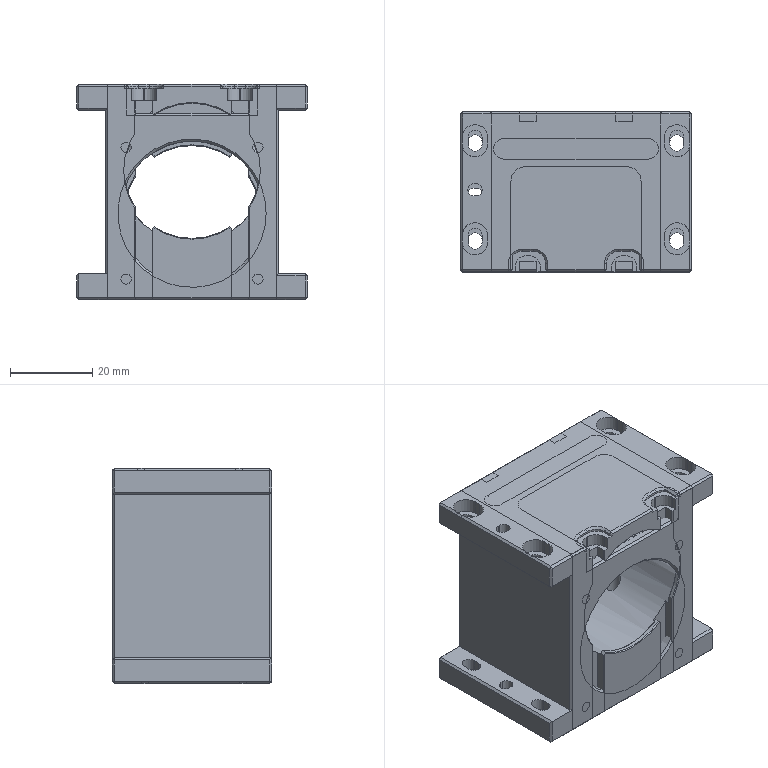Part | 2 solids | 662 faces | box 56 x 38.8 x 52.3 mm | volume 86600 mm3 | plane 450 | cylinder 126 | cone 54 | spline 32 | commonest cylinder face diameters 6 x20 3.4 x16 6.2 x16 2.5 x8 3 x8 32.8 x8